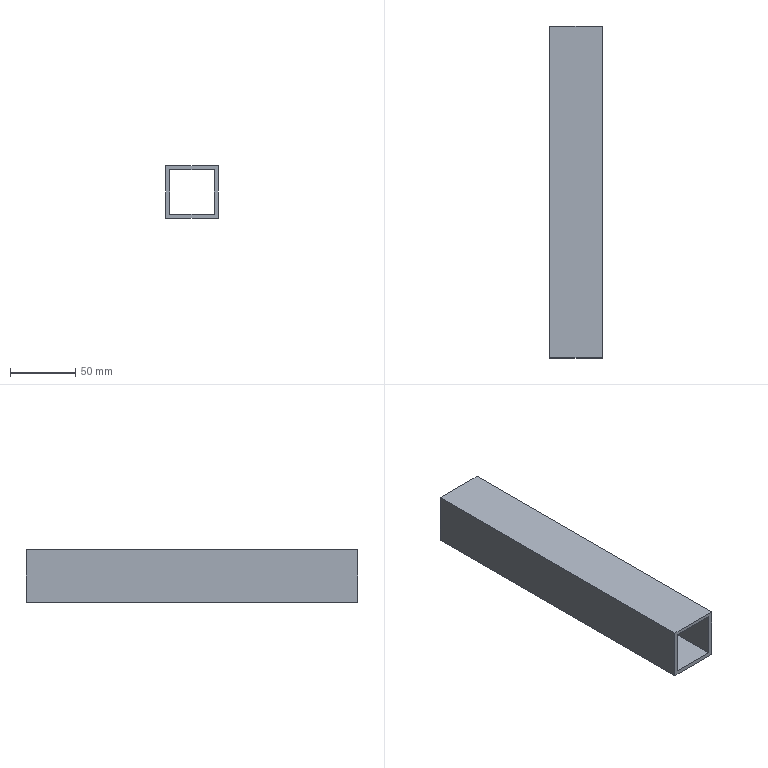Part | STEP file | Guide wheel mechanism revised.sldasm-Part-65 | 1 solid | 10 faces | box 40 x 255 x 40 mm | volume 113220 mm3 | plane 10
STEP:
#1=CARTESIAN_POINT('',(-443.5,255.,20.));
#2=VERTEX_POINT('',#1);
#3=CARTESIAN_POINT('',(-443.5,255.,-20.));
#4=VERTEX_POINT('',#3);
#5=CARTESIAN_POINT('',(-443.5,255.,20.));
#6=DIRECTION('',(0.,0.,-1.));
#7=VECTOR('',#6,1000.);
#8=LINE('',#5,#7);
#9=EDGE_CURVE('',#2,#4,#8,.T.);
#10=ORIENTED_EDGE('',*,*,#9,.T.);
#11=CARTESIAN_POINT('',(-483.5,255.,-20.));
#12=VERTEX_POINT('',#11);
#13=CARTESIAN_POINT('',(-483.5,255.,-20.));
#14=DIRECTION('',(-1.,0.,0.));
#15=VECTOR('',#14,1000.);
#16=LINE('',#13,#15);
#17=EDGE_CURVE('',#4,#12,#16,.T.);
#18=ORIENTED_EDGE('',*,*,#17,.T.);
#19=CARTESIAN_POINT('',(-483.5,255.,20.));
#20=VERTEX_POINT('',#19);
#21=CARTESIAN_POINT('',(-483.5,255.,20.));
#22=DIRECTION('',(0.,0.,1.));
#23=VECTOR('',#22,1000.);
#24=LINE('',#21,#23);
#25=EDGE_CURVE('',#12,#20,#24,.T.);
#26=ORIENTED_EDGE('',*,*,#25,.T.);
#27=CARTESIAN_POINT('',(-483.5,255.,20.));
#28=DIRECTION('',(1.,0.,0.));
#29=VECTOR('',#28,1000.);
#30=LINE('',#27,#29);
#31=EDGE_CURVE('',#20,#2,#30,.T.);
#32=ORIENTED_EDGE('',*,*,#31,.T.);
#33=EDGE_LOOP('',(#10,#18,#26,#32));
#34=FACE_OUTER_BOUND('',#33,.T.);
#35=CARTESIAN_POINT('',(-480.5,255.,-17.));
#36=VERTEX_POINT('',#35);
#37=CARTESIAN_POINT('',(-480.5,255.,17.));
#38=VERTEX_POINT('',#37);
#39=CARTESIAN_POINT('',(-480.5,255.,17.));
#40=DIRECTION('',(0.,0.,1.));
#41=VECTOR('',#40,1000.);
#42=LINE('',#39,#41);
#43=EDGE_CURVE('',#36,#38,#42,.T.);
#44=ORIENTED_EDGE('',*,*,#43,.F.);
#45=CARTESIAN_POINT('',(-446.5,255.,-17.));
#46=VERTEX_POINT('',#45);
#47=CARTESIAN_POINT('',(-480.5,255.,-17.));
#48=DIRECTION('',(-1.,0.,0.));
#49=VECTOR('',#48,1000.);
#50=LINE('',#47,#49);
#51=EDGE_CURVE('',#46,#36,#50,.T.);
#52=ORIENTED_EDGE('',*,*,#51,.F.);
#53=CARTESIAN_POINT('',(-446.5,255.,17.));
#54=VERTEX_POINT('',#53);
#55=CARTESIAN_POINT('',(-446.5,255.,17.));
#56=DIRECTION('',(0.,0.,-1.));
#57=VECTOR('',#56,1000.);
#58=LINE('',#55,#57);
#59=EDGE_CURVE('',#54,#46,#58,.T.);
#60=ORIENTED_EDGE('',*,*,#59,.F.);
#61=CARTESIAN_POINT('',(-480.5,255.,17.));
#62=DIRECTION('',(1.,0.,0.));
#63=VECTOR('',#62,1000.);
#64=LINE('',#61,#63);
#65=EDGE_CURVE('',#38,#54,#64,.T.);
#66=ORIENTED_EDGE('',*,*,#65,.F.);
#67=EDGE_LOOP('',(#44,#52,#60,#66));
#68=FACE_BOUND('',#67,.T.);
#69=CARTESIAN_POINT('',(0.,255.,0.));
#70=DIRECTION('',(0.,-1.,0.));
#71=DIRECTION('',(0.,0.,-1.));
#72=AXIS2_PLACEMENT_3D('',#69,#70,#71);
#73=PLANE('',#72);
#74=ADVANCED_FACE('',(#34,#68),#73,.F.);
#75=CARTESIAN_POINT('',(-443.5,0.,20.));
#76=VERTEX_POINT('',#75);
#77=CARTESIAN_POINT('',(-443.5,0.,-20.));
#78=VERTEX_POINT('',#77);
#79=CARTESIAN_POINT('',(-443.5,0.,20.));
#80=DIRECTION('',(0.,0.,-1.));
#81=VECTOR('',#80,1000.);
#82=LINE('',#79,#81);
#83=EDGE_CURVE('',#76,#78,#82,.T.);
#84=ORIENTED_EDGE('',*,*,#83,.F.);
#85=CARTESIAN_POINT('',(-483.5,0.,20.));
#86=VERTEX_POINT('',#85);
#87=CARTESIAN_POINT('',(-483.5,0.,20.));
#88=DIRECTION('',(1.,0.,0.));
#89=VECTOR('',#88,1000.);
#90=LINE('',#87,#89);
#91=EDGE_CURVE('',#86,#76,#90,.T.);
#92=ORIENTED_EDGE('',*,*,#91,.F.);
#93=CARTESIAN_POINT('',(-483.5,0.,-20.));
#94=VERTEX_POINT('',#93);
#95=CARTESIAN_POINT('',(-483.5,0.,20.));
#96=DIRECTION('',(0.,0.,1.));
#97=VECTOR('',#96,1000.);
#98=LINE('',#95,#97);
#99=EDGE_CURVE('',#94,#86,#98,.T.);
#100=ORIENTED_EDGE('',*,*,#99,.F.);
#101=CARTESIAN_POINT('',(-483.5,0.,-20.));
#102=DIRECTION('',(-1.,0.,0.));
#103=VECTOR('',#102,1000.);
#104=LINE('',#101,#103);
#105=EDGE_CURVE('',#78,#94,#104,.T.);
#106=ORIENTED_EDGE('',*,*,#105,.F.);
#107=EDGE_LOOP('',(#84,#92,#100,#106));
#108=FACE_OUTER_BOUND('',#107,.T.);
#109=CARTESIAN_POINT('',(-446.5,0.,-17.));
#110=VERTEX_POINT('',#109);
#111=CARTESIAN_POINT('',(-480.5,0.,-17.));
#112=VERTEX_POINT('',#111);
#113=CARTESIAN_POINT('',(-480.5,0.,-17.));
#114=DIRECTION('',(-1.,0.,0.));
#115=VECTOR('',#114,1000.);
#116=LINE('',#113,#115);
#117=EDGE_CURVE('',#110,#112,#116,.T.);
#118=ORIENTED_EDGE('',*,*,#117,.T.);
#119=CARTESIAN_POINT('',(-480.5,0.,17.));
#120=VERTEX_POINT('',#119);
#121=CARTESIAN_POINT('',(-480.5,0.,17.));
#122=DIRECTION('',(0.,0.,1.));
#123=VECTOR('',#122,1000.);
#124=LINE('',#121,#123);
#125=EDGE_CURVE('',#112,#120,#124,.T.);
#126=ORIENTED_EDGE('',*,*,#125,.T.);
#127=CARTESIAN_POINT('',(-446.5,0.,17.));
#128=VERTEX_POINT('',#127);
#129=CARTESIAN_POINT('',(-480.5,0.,17.));
#130=DIRECTION('',(1.,0.,0.));
#131=VECTOR('',#130,1000.);
#132=LINE('',#129,#131);
#133=EDGE_CURVE('',#120,#128,#132,.T.);
#134=ORIENTED_EDGE('',*,*,#133,.T.);
#135=CARTESIAN_POINT('',(-446.5,0.,17.));
#136=DIRECTION('',(0.,0.,-1.));
#137=VECTOR('',#136,1000.);
#138=LINE('',#135,#137);
#139=EDGE_CURVE('',#128,#110,#138,.T.);
#140=ORIENTED_EDGE('',*,*,#139,.T.);
#141=EDGE_LOOP('',(#118,#126,#134,#140));
#142=FACE_BOUND('',#141,.T.);
#143=CARTESIAN_POINT('',(0.,0.,0.));
#144=DIRECTION('',(0.,-1.,0.));
#145=DIRECTION('',(0.,0.,-1.));
#146=AXIS2_PLACEMENT_3D('',#143,#144,#145);
#147=PLANE('',#146);
#148=ADVANCED_FACE('',(#108,#142),#147,.T.);
#149=ORIENTED_EDGE('',*,*,#83,.T.);
#150=CARTESIAN_POINT('',(-443.5,255.,-20.));
#151=DIRECTION('',(0.,-1.,0.));
#152=VECTOR('',#151,1000.);
#153=LINE('',#150,#152);
#154=EDGE_CURVE('',#4,#78,#153,.T.);
#155=ORIENTED_EDGE('',*,*,#154,.F.);
#156=ORIENTED_EDGE('',*,*,#9,.F.);
#157=CARTESIAN_POINT('',(-443.5,255.,20.));
#158=DIRECTION('',(0.,-1.,0.));
#159=VECTOR('',#158,1000.);
#160=LINE('',#157,#159);
#161=EDGE_CURVE('',#2,#76,#160,.T.);
#162=ORIENTED_EDGE('',*,*,#161,.T.);
#163=EDGE_LOOP('',(#149,#155,#156,#162));
#164=FACE_OUTER_BOUND('',#163,.T.);
#165=CARTESIAN_POINT('',(-443.5,255.,20.));
#166=DIRECTION('',(-1.,0.,0.));
#167=DIRECTION('',(0.,0.,1.));
#168=AXIS2_PLACEMENT_3D('',#165,#166,#167);
#169=PLANE('',#168);
#170=ADVANCED_FACE('',(#164),#169,.F.);
#171=ORIENTED_EDGE('',*,*,#105,.T.);
#172=CARTESIAN_POINT('',(-483.5,255.,-20.));
#173=DIRECTION('',(0.,-1.,0.));
#174=VECTOR('',#173,1000.);
#175=LINE('',#172,#174);
#176=EDGE_CURVE('',#12,#94,#175,.T.);
#177=ORIENTED_EDGE('',*,*,#176,.F.);
#178=ORIENTED_EDGE('',*,*,#17,.F.);
#179=ORIENTED_EDGE('',*,*,#154,.T.);
#180=EDGE_LOOP('',(#171,#177,#178,#179));
#181=FACE_OUTER_BOUND('',#180,.T.);
#182=CARTESIAN_POINT('',(-483.5,255.,-20.));
#183=DIRECTION('',(0.,0.,1.));
#184=DIRECTION('',(1.,0.,0.));
#185=AXIS2_PLACEMENT_3D('',#182,#183,#184);
#186=PLANE('',#185);
#187=ADVANCED_FACE('',(#181),#186,.F.);
#188=ORIENTED_EDGE('',*,*,#99,.T.);
#189=CARTESIAN_POINT('',(-483.5,255.,20.));
#190=DIRECTION('',(0.,-1.,0.));
#191=VECTOR('',#190,1000.);
#192=LINE('',#189,#191);
#193=EDGE_CURVE('',#20,#86,#192,.T.);
#194=ORIENTED_EDGE('',*,*,#193,.F.);
#195=ORIENTED_EDGE('',*,*,#25,.F.);
#196=ORIENTED_EDGE('',*,*,#176,.T.);
#197=EDGE_LOOP('',(#188,#194,#195,#196));
#198=FACE_OUTER_BOUND('',#197,.T.);
#199=CARTESIAN_POINT('',(-483.5,255.,20.));
#200=DIRECTION('',(1.,0.,0.));
#201=DIRECTION('',(0.,0.,-1.));
#202=AXIS2_PLACEMENT_3D('',#199,#200,#201);
#203=PLANE('',#202);
#204=ADVANCED_FACE('',(#198),#203,.F.);
#205=ORIENTED_EDGE('',*,*,#91,.T.);
#206=ORIENTED_EDGE('',*,*,#161,.F.);
#207=ORIENTED_EDGE('',*,*,#31,.F.);
#208=ORIENTED_EDGE('',*,*,#193,.T.);
#209=EDGE_LOOP('',(#205,#206,#207,#208));
#210=FACE_OUTER_BOUND('',#209,.T.);
#211=CARTESIAN_POINT('',(-483.5,255.,20.));
#212=DIRECTION('',(0.,0.,-1.));
#213=DIRECTION('',(-1.,0.,0.));
#214=AXIS2_PLACEMENT_3D('',#211,#212,#213);
#215=PLANE('',#214);
#216=ADVANCED_FACE('',(#210),#215,.F.);
#217=ORIENTED_EDGE('',*,*,#125,.F.);
#218=CARTESIAN_POINT('',(-480.5,255.,-17.));
#219=DIRECTION('',(0.,-1.,0.));
#220=VECTOR('',#219,1000.);
#221=LINE('',#218,#220);
#222=EDGE_CURVE('',#36,#112,#221,.T.);
#223=ORIENTED_EDGE('',*,*,#222,.F.);
#224=ORIENTED_EDGE('',*,*,#43,.T.);
#225=CARTESIAN_POINT('',(-480.5,255.,17.));
#226=DIRECTION('',(0.,-1.,0.));
#227=VECTOR('',#226,1000.);
#228=LINE('',#225,#227);
#229=EDGE_CURVE('',#38,#120,#228,.T.);
#230=ORIENTED_EDGE('',*,*,#229,.T.);
#231=EDGE_LOOP('',(#217,#223,#224,#230));
#232=FACE_OUTER_BOUND('',#231,.T.);
#233=CARTESIAN_POINT('',(-480.5,255.,17.));
#234=DIRECTION('',(1.,0.,0.));
#235=DIRECTION('',(0.,0.,-1.));
#236=AXIS2_PLACEMENT_3D('',#233,#234,#235);
#237=PLANE('',#236);
#238=ADVANCED_FACE('',(#232),#237,.T.);
#239=ORIENTED_EDGE('',*,*,#133,.F.);
#240=ORIENTED_EDGE('',*,*,#229,.F.);
#241=ORIENTED_EDGE('',*,*,#65,.T.);
#242=CARTESIAN_POINT('',(-446.5,255.,17.));
#243=DIRECTION('',(0.,-1.,0.));
#244=VECTOR('',#243,1000.);
#245=LINE('',#242,#244);
#246=EDGE_CURVE('',#54,#128,#245,.T.);
#247=ORIENTED_EDGE('',*,*,#246,.T.);
#248=EDGE_LOOP('',(#239,#240,#241,#247));
#249=FACE_OUTER_BOUND('',#248,.T.);
#250=CARTESIAN_POINT('',(-480.5,255.,17.));
#251=DIRECTION('',(0.,0.,-1.));
#252=DIRECTION('',(-1.,0.,0.));
#253=AXIS2_PLACEMENT_3D('',#250,#251,#252);
#254=PLANE('',#253);
#255=ADVANCED_FACE('',(#249),#254,.T.);
#256=ORIENTED_EDGE('',*,*,#139,.F.);
#257=ORIENTED_EDGE('',*,*,#246,.F.);
#258=ORIENTED_EDGE('',*,*,#59,.T.);
#259=CARTESIAN_POINT('',(-446.5,255.,-17.));
#260=DIRECTION('',(0.,-1.,0.));
#261=VECTOR('',#260,1000.);
#262=LINE('',#259,#261);
#263=EDGE_CURVE('',#46,#110,#262,.T.);
#264=ORIENTED_EDGE('',*,*,#263,.T.);
#265=EDGE_LOOP('',(#256,#257,#258,#264));
#266=FACE_OUTER_BOUND('',#265,.T.);
#267=CARTESIAN_POINT('',(-446.5,255.,17.));
#268=DIRECTION('',(-1.,0.,0.));
#269=DIRECTION('',(0.,0.,1.));
#270=AXIS2_PLACEMENT_3D('',#267,#268,#269);
#271=PLANE('',#270);
#272=ADVANCED_FACE('',(#266),#271,.T.);
#273=ORIENTED_EDGE('',*,*,#117,.F.);
#274=ORIENTED_EDGE('',*,*,#263,.F.);
#275=ORIENTED_EDGE('',*,*,#51,.T.);
#276=ORIENTED_EDGE('',*,*,#222,.T.);
#277=EDGE_LOOP('',(#273,#274,#275,#276));
#278=FACE_OUTER_BOUND('',#277,.T.);
#279=CARTESIAN_POINT('',(-480.5,255.,-17.));
#280=DIRECTION('',(0.,0.,1.));
#281=DIRECTION('',(1.,0.,0.));
#282=AXIS2_PLACEMENT_3D('',#279,#280,#281);
#283=PLANE('',#282);
#284=ADVANCED_FACE('',(#278),#283,.T.);
#285=CLOSED_SHELL('',(#74,#148,#170,#187,#204,#216,#238,#255,#272,#284));
#286=MANIFOLD_SOLID_BREP('',#285);
#287=CARTESIAN_POINT('',(0.,0.,0.));
#288=DIRECTION('',(0.,0.,1.));
#289=DIRECTION('',(1.,0.,0.));
#290=AXIS2_PLACEMENT_3D('',#287,#288,#289);
#291=(LENGTH_UNIT()NAMED_UNIT(*)SI_UNIT(.MILLI.,.METRE.));
#292=UNCERTAINTY_MEASURE_WITH_UNIT(LENGTH_MEASURE(0.00001),#291,'','');
#293=(NAMED_UNIT(*)PLANE_ANGLE_UNIT()SI_UNIT($,.RADIAN.));
#294=(NAMED_UNIT(*)SI_UNIT($,.STERADIAN.)SOLID_ANGLE_UNIT());
#295=(GEOMETRIC_REPRESENTATION_CONTEXT(3)GLOBAL_UNCERTAINTY_ASSIGNED_CONTEXT((#292))GLOBAL_UNIT_ASSIGNED_CONTEXT((#291,#293,#294))REPRESENTATION_CONTEXT('',''));
#296=ADVANCED_BREP_SHAPE_REPRESENTATION('',(#286,#290),#295);